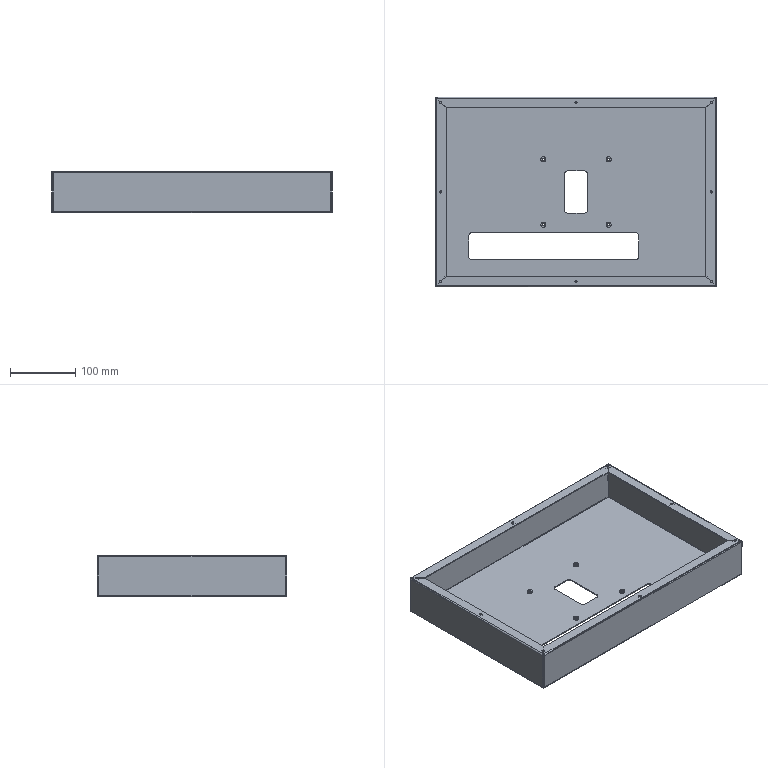Part | SolidWorks | features ICE 4, SMWeldBead 4, EdgeFlange 2, HoleWzd 2, FlatPattern 1, SMBaseFlange 1, SheetMetal 1 | 1 solid | 198 faces | box 430 x 290 x 63 mm | volume 327890 mm3 | plane 82 | cylinder 76 | spline 40 | commonest cylinder face diameters 3.3 x24 8 x24 1 x8 4 x8 10 x8 2 x4